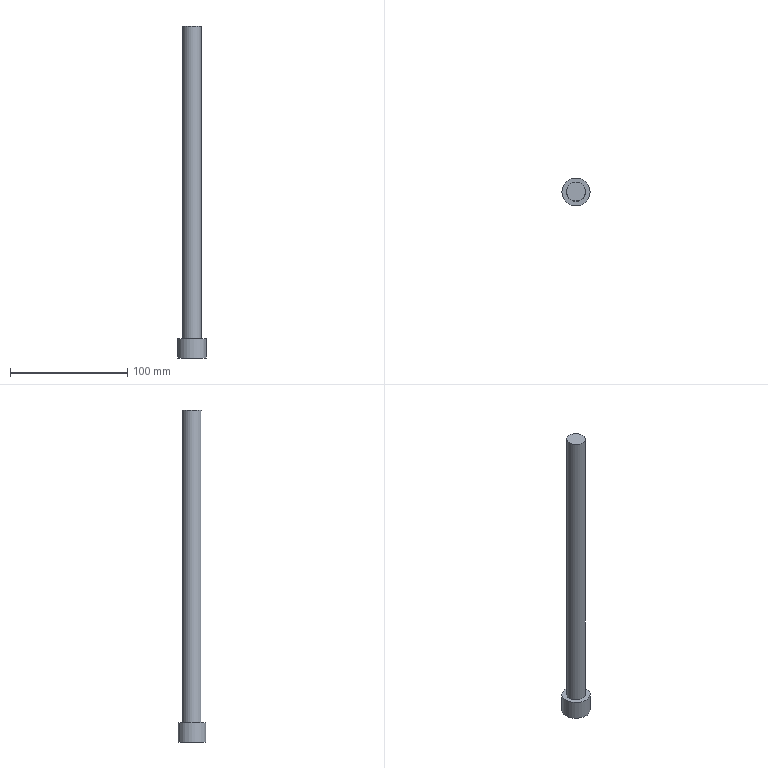Part | STEP file | solid 25 | 1 solid | 12 faces | box 24 x 24 x 283.5 mm | volume 59748 mm3 | plane 10 | cylinder 2 | commonest cylinder face diameters 16 x1 24 x1